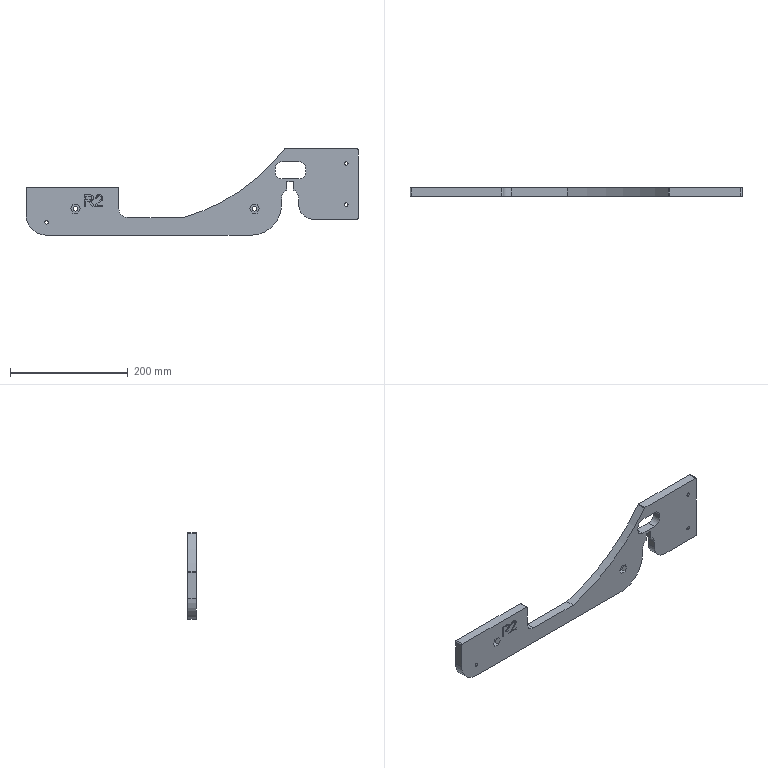Part | STEP file | Right | 1 solid | 106 faces | box 565 x 15 x 147 mm | volume 597493 mm3 | plane 51 | other 34 | cylinder 21 | commonest cylinder face diameters 4 x5 24 x4 6 x3 8 x2 29 x2 30 x1